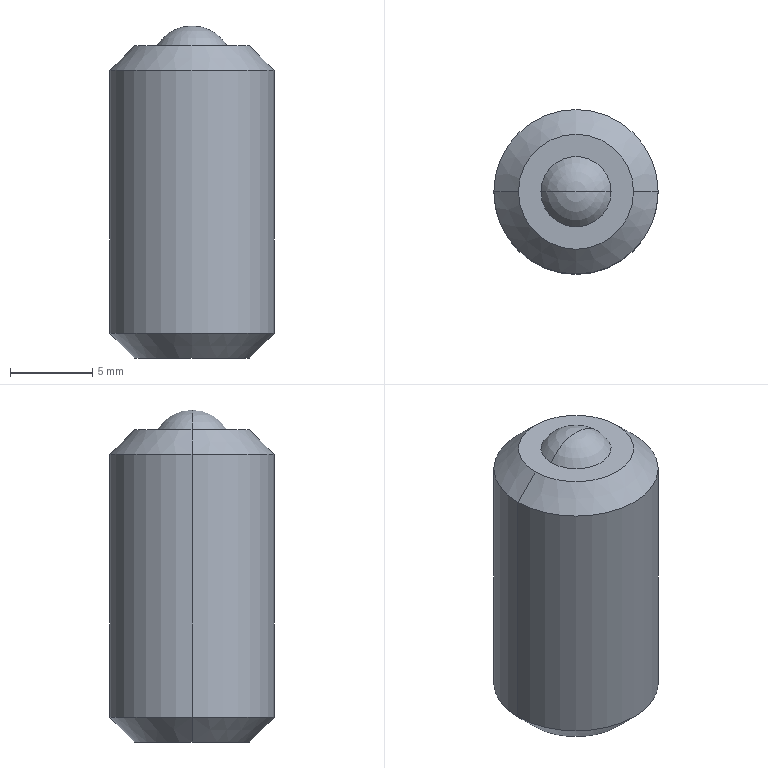Part | Creo | 1 solid | 17 faces | box 10 x 10 x 20.2 mm | volume 1251 mm3 | plane 9 | cone 4 | cylinder 2 | sphere 2 | commonest cylinder face diameters 10 x2
STEP:
#1=CARTESIAN_POINT('',(-220.5,-57.908,-54.5));
#2=VERTEX_POINT('',#1);
#3=CARTESIAN_POINT('',(-213.5,-57.908,-54.5));
#4=VERTEX_POINT('',#3);
#5=CARTESIAN_POINT('',(-217.,-57.908,-54.5));
#6=DIRECTION('',(0.,0.,-1.));
#7=DIRECTION('',(-1.,0.,0.));
#8=AXIS2_PLACEMENT_3D('',#5,#6,#7);
#9=CIRCLE('',#8,3.5);
#10=EDGE_CURVE('',#2,#4,#9,.T.);
#11=ORIENTED_EDGE('',*,*,#10,.F.);
#12=CARTESIAN_POINT('',(-217.,-57.908,-54.5));
#13=DIRECTION('',(0.,0.,-1.));
#14=DIRECTION('',(1.,0.,0.));
#15=AXIS2_PLACEMENT_3D('',#12,#13,#14);
#16=CIRCLE('',#15,3.5);
#17=EDGE_CURVE('',#4,#2,#16,.T.);
#18=ORIENTED_EDGE('',*,*,#17,.F.);
#19=EDGE_LOOP('',(#11,#18));
#20=FACE_OUTER_BOUND('',#19,.F.);
#21=CARTESIAN_POINT('',(-220.,-59.64,-54.5));
#22=VERTEX_POINT('',#21);
#23=CARTESIAN_POINT('',(-217.,-61.372,-54.5));
#24=VERTEX_POINT('',#23);
#25=CARTESIAN_POINT('',(-220.,-59.64,-54.5));
#26=DIRECTION('',(0.866,-0.5,0.));
#27=VECTOR('',#26,3.464);
#28=LINE('',#25,#27);
#29=EDGE_CURVE('',#22,#24,#28,.T.);
#30=ORIENTED_EDGE('',*,*,#29,.F.);
#31=CARTESIAN_POINT('',(-220.,-56.176,-54.5));
#32=VERTEX_POINT('',#31);
#33=CARTESIAN_POINT('',(-220.,-59.64,-54.5));
#34=DIRECTION('',(0.,1.,0.));
#35=VECTOR('',#34,3.464);
#36=LINE('',#33,#35);
#37=EDGE_CURVE('',#22,#32,#36,.T.);
#38=ORIENTED_EDGE('',*,*,#37,.T.);
#39=CARTESIAN_POINT('',(-217.,-54.444,-54.5));
#40=VERTEX_POINT('',#39);
#41=CARTESIAN_POINT('',(-217.,-54.444,-54.5));
#42=DIRECTION('',(-0.866,-0.5,0.));
#43=VECTOR('',#42,3.464);
#44=LINE('',#41,#43);
#45=EDGE_CURVE('',#40,#32,#44,.T.);
#46=ORIENTED_EDGE('',*,*,#45,.F.);
#47=CARTESIAN_POINT('',(-214.,-56.176,-54.5));
#48=VERTEX_POINT('',#47);
#49=CARTESIAN_POINT('',(-214.,-56.176,-54.5));
#50=DIRECTION('',(-0.866,0.5,0.));
#51=VECTOR('',#50,3.464);
#52=LINE('',#49,#51);
#53=EDGE_CURVE('',#48,#40,#52,.T.);
#54=ORIENTED_EDGE('',*,*,#53,.F.);
#55=CARTESIAN_POINT('',(-214.,-59.64,-54.5));
#56=VERTEX_POINT('',#55);
#57=CARTESIAN_POINT('',(-214.,-56.176,-54.5));
#58=DIRECTION('',(0.,-1.,0.));
#59=VECTOR('',#58,3.464);
#60=LINE('',#57,#59);
#61=EDGE_CURVE('',#48,#56,#60,.T.);
#62=ORIENTED_EDGE('',*,*,#61,.T.);
#63=CARTESIAN_POINT('',(-217.,-61.372,-54.5));
#64=DIRECTION('',(0.866,0.5,0.));
#65=VECTOR('',#64,3.464);
#66=LINE('',#63,#65);
#67=EDGE_CURVE('',#24,#56,#66,.T.);
#68=ORIENTED_EDGE('',*,*,#67,.F.);
#69=EDGE_LOOP('',(#30,#38,#46,#54,#62,#68));
#70=FACE_BOUND('',#69,.F.);
#71=CARTESIAN_POINT('',(-217.,-57.908,-54.5));
#72=DIRECTION('',(0.,0.,-1.));
#73=DIRECTION('',(-1.,0.,0.));
#74=AXIS2_PLACEMENT_3D('',#71,#72,#73);
#75=PLANE('',#74);
#76=ADVANCED_FACE('',(#20,#70),#75,.T.);
#77=ORIENTED_EDGE('',*,*,#10,.T.);
#78=CARTESIAN_POINT('',(-212.,-57.908,-53.));
#79=VERTEX_POINT('',#78);
#80=CARTESIAN_POINT('',(-213.5,-57.908,-54.5));
#81=DIRECTION('',(0.7071,0.,0.7071));
#82=VECTOR('',#81,2.121);
#83=LINE('',#80,#82);
#84=EDGE_CURVE('',#4,#79,#83,.T.);
#85=ORIENTED_EDGE('',*,*,#84,.T.);
#86=CARTESIAN_POINT('',(-222.,-57.908,-53.));
#87=VERTEX_POINT('',#86);
#88=CARTESIAN_POINT('',(-217.,-57.908,-53.));
#89=DIRECTION('',(0.,0.,-1.));
#90=DIRECTION('',(-1.,0.,0.));
#91=AXIS2_PLACEMENT_3D('',#88,#89,#90);
#92=CIRCLE('',#91,5.);
#93=EDGE_CURVE('',#87,#79,#92,.T.);
#94=ORIENTED_EDGE('',*,*,#93,.F.);
#95=CARTESIAN_POINT('',(-220.5,-57.908,-54.5));
#96=DIRECTION('',(-0.7071,0.,0.7071));
#97=VECTOR('',#96,2.121);
#98=LINE('',#95,#97);
#99=EDGE_CURVE('',#2,#87,#98,.T.);
#100=ORIENTED_EDGE('',*,*,#99,.F.);
#101=EDGE_LOOP('',(#77,#85,#94,#100));
#102=FACE_OUTER_BOUND('',#101,.F.);
#103=CARTESIAN_POINT('',(-217.,-57.908,-53.75));
#104=DIRECTION('',(0.,0.,1.));
#105=DIRECTION('',(1.,0.,0.));
#106=AXIS2_PLACEMENT_3D('',#103,#104,#105);
#107=CONICAL_SURFACE('',#106,4.25,45.);
#108=ADVANCED_FACE('',(#102),#107,.T.);
#109=ORIENTED_EDGE('',*,*,#17,.T.);
#110=ORIENTED_EDGE('',*,*,#99,.T.);
#111=CARTESIAN_POINT('',(-217.,-57.908,-53.));
#112=DIRECTION('',(0.,0.,-1.));
#113=DIRECTION('',(1.,0.,0.));
#114=AXIS2_PLACEMENT_3D('',#111,#112,#113);
#115=CIRCLE('',#114,5.);
#116=EDGE_CURVE('',#79,#87,#115,.T.);
#117=ORIENTED_EDGE('',*,*,#116,.F.);
#118=ORIENTED_EDGE('',*,*,#84,.F.);
#119=EDGE_LOOP('',(#109,#110,#117,#118));
#120=FACE_OUTER_BOUND('',#119,.F.);
#121=CARTESIAN_POINT('',(-217.,-57.908,-53.75));
#122=DIRECTION('',(0.,0.,1.));
#123=DIRECTION('',(1.,0.,0.));
#124=AXIS2_PLACEMENT_3D('',#121,#122,#123);
#125=CONICAL_SURFACE('',#124,4.25,45.);
#126=ADVANCED_FACE('',(#120),#125,.T.);
#127=ORIENTED_EDGE('',*,*,#116,.T.);
#128=CARTESIAN_POINT('',(-222.,-57.908,-37.));
#129=VERTEX_POINT('',#128);
#130=CARTESIAN_POINT('',(-222.,-57.908,-37.));
#131=DIRECTION('',(0.,0.,-1.));
#132=VECTOR('',#131,16.);
#133=LINE('',#130,#132);
#134=EDGE_CURVE('',#129,#87,#133,.T.);
#135=ORIENTED_EDGE('',*,*,#134,.F.);
#136=CARTESIAN_POINT('',(-212.,-57.908,-37.));
#137=VERTEX_POINT('',#136);
#138=CARTESIAN_POINT('',(-217.,-57.908,-37.));
#139=DIRECTION('',(0.,0.,1.));
#140=DIRECTION('',(-1.,0.,0.));
#141=AXIS2_PLACEMENT_3D('',#138,#139,#140);
#142=CIRCLE('',#141,5.);
#143=EDGE_CURVE('',#129,#137,#142,.T.);
#144=ORIENTED_EDGE('',*,*,#143,.T.);
#145=CARTESIAN_POINT('',(-212.,-57.908,-37.));
#146=DIRECTION('',(0.,0.,-1.));
#147=VECTOR('',#146,16.);
#148=LINE('',#145,#147);
#149=EDGE_CURVE('',#137,#79,#148,.T.);
#150=ORIENTED_EDGE('',*,*,#149,.T.);
#151=EDGE_LOOP('',(#127,#135,#144,#150));
#152=FACE_OUTER_BOUND('',#151,.F.);
#153=CARTESIAN_POINT('',(-217.,-57.908,-35.5));
#154=DIRECTION('',(0.,0.,-1.));
#155=DIRECTION('',(-1.,0.,0.));
#156=AXIS2_PLACEMENT_3D('',#153,#154,#155);
#157=CYLINDRICAL_SURFACE('',#156,5.);
#158=ADVANCED_FACE('',(#152),#157,.T.);
#159=ORIENTED_EDGE('',*,*,#93,.T.);
#160=ORIENTED_EDGE('',*,*,#149,.F.);
#161=CARTESIAN_POINT('',(-217.,-57.908,-37.));
#162=DIRECTION('',(0.,0.,1.));
#163=DIRECTION('',(1.,0.,0.));
#164=AXIS2_PLACEMENT_3D('',#161,#162,#163);
#165=CIRCLE('',#164,5.);
#166=EDGE_CURVE('',#137,#129,#165,.T.);
#167=ORIENTED_EDGE('',*,*,#166,.T.);
#168=ORIENTED_EDGE('',*,*,#134,.T.);
#169=EDGE_LOOP('',(#159,#160,#167,#168));
#170=FACE_OUTER_BOUND('',#169,.F.);
#171=CARTESIAN_POINT('',(-217.,-57.908,-35.5));
#172=DIRECTION('',(0.,0.,-1.));
#173=DIRECTION('',(-1.,0.,0.));
#174=AXIS2_PLACEMENT_3D('',#171,#172,#173);
#175=CYLINDRICAL_SURFACE('',#174,5.);
#176=ADVANCED_FACE('',(#170),#175,.T.);
#177=CARTESIAN_POINT('',(-213.5,-57.908,-35.5));
#178=VERTEX_POINT('',#177);
#179=CARTESIAN_POINT('',(-220.5,-57.908,-35.5));
#180=VERTEX_POINT('',#179);
#181=CARTESIAN_POINT('',(-217.,-57.908,-35.5));
#182=DIRECTION('',(0.,0.,1.));
#183=DIRECTION('',(1.,0.,0.));
#184=AXIS2_PLACEMENT_3D('',#181,#182,#183);
#185=CIRCLE('',#184,3.5);
#186=EDGE_CURVE('',#178,#180,#185,.T.);
#187=ORIENTED_EDGE('',*,*,#186,.T.);
#188=CARTESIAN_POINT('',(-220.5,-57.908,-35.5));
#189=DIRECTION('',(-0.7071,0.,-0.7071));
#190=VECTOR('',#189,2.121);
#191=LINE('',#188,#190);
#192=EDGE_CURVE('',#180,#129,#191,.T.);
#193=ORIENTED_EDGE('',*,*,#192,.T.);
#194=ORIENTED_EDGE('',*,*,#166,.F.);
#195=CARTESIAN_POINT('',(-213.5,-57.908,-35.5));
#196=DIRECTION('',(0.7071,0.,-0.7071));
#197=VECTOR('',#196,2.121);
#198=LINE('',#195,#197);
#199=EDGE_CURVE('',#178,#137,#198,.T.);
#200=ORIENTED_EDGE('',*,*,#199,.F.);
#201=EDGE_LOOP('',(#187,#193,#194,#200));
#202=FACE_OUTER_BOUND('',#201,.F.);
#203=CARTESIAN_POINT('',(-217.,-57.908,-36.25));
#204=DIRECTION('',(0.,0.,-1.));
#205=DIRECTION('',(-1.,0.,0.));
#206=AXIS2_PLACEMENT_3D('',#203,#204,#205);
#207=CONICAL_SURFACE('',#206,4.25,45.);
#208=ADVANCED_FACE('',(#202),#207,.T.);
#209=ORIENTED_EDGE('',*,*,#186,.F.);
#210=CARTESIAN_POINT('',(-217.,-57.908,-35.5));
#211=DIRECTION('',(0.,0.,1.));
#212=DIRECTION('',(-1.,0.,0.));
#213=AXIS2_PLACEMENT_3D('',#210,#211,#212);
#214=CIRCLE('',#213,3.5);
#215=EDGE_CURVE('',#180,#178,#214,.T.);
#216=ORIENTED_EDGE('',*,*,#215,.F.);
#217=EDGE_LOOP('',(#209,#216));
#218=FACE_OUTER_BOUND('',#217,.F.);
#219=CARTESIAN_POINT('',(-214.865,-57.908,-35.5));
#220=VERTEX_POINT('',#219);
#221=CARTESIAN_POINT('',(-219.135,-57.908,-35.5));
#222=VERTEX_POINT('',#221);
#223=CARTESIAN_POINT('',(-217.,-57.908,-35.5));
#224=DIRECTION('',(0.,0.,-1.));
#225=DIRECTION('',(1.,0.,0.));
#226=AXIS2_PLACEMENT_3D('',#223,#224,#225);
#227=CIRCLE('',#226,2.135);
#228=EDGE_CURVE('',#220,#222,#227,.T.);
#229=ORIENTED_EDGE('',*,*,#228,.F.);
#230=CARTESIAN_POINT('',(-217.,-57.908,-35.5));
#231=DIRECTION('',(0.,0.,-1.));
#232=DIRECTION('',(-1.,0.,0.));
#233=AXIS2_PLACEMENT_3D('',#230,#231,#232);
#234=CIRCLE('',#233,2.135);
#235=EDGE_CURVE('',#222,#220,#234,.T.);
#236=ORIENTED_EDGE('',*,*,#235,.F.);
#237=EDGE_LOOP('',(#229,#236));
#238=FACE_BOUND('',#237,.F.);
#239=CARTESIAN_POINT('',(-217.,-57.908,-35.5));
#240=DIRECTION('',(0.,0.,1.));
#241=DIRECTION('',(1.,0.,0.));
#242=AXIS2_PLACEMENT_3D('',#239,#240,#241);
#243=PLANE('',#242);
#244=ADVANCED_FACE('',(#218,#238),#243,.T.);
#245=ORIENTED_EDGE('',*,*,#228,.T.);
#246=CARTESIAN_POINT('',(-217.,-57.908,-34.3));
#247=VERTEX_POINT('',#246);
#248=CARTESIAN_POINT('',(-217.,-57.908,-36.8));
#249=DIRECTION('',(0.,1.,0.));
#250=DIRECTION('',(-0.8542,0.,0.52));
#251=AXIS2_PLACEMENT_3D('',#248,#249,#250);
#252=CIRCLE('',#251,2.5);
#253=EDGE_CURVE('',#222,#247,#252,.T.);
#254=ORIENTED_EDGE('',*,*,#253,.T.);
#255=CARTESIAN_POINT('',(-217.,-57.908,-36.8));
#256=DIRECTION('',(0.,-1.,0.));
#257=DIRECTION('',(0.8542,0.,0.52));
#258=AXIS2_PLACEMENT_3D('',#255,#256,#257);
#259=CIRCLE('',#258,2.5);
#260=EDGE_CURVE('',#220,#247,#259,.T.);
#261=ORIENTED_EDGE('',*,*,#260,.F.);
#262=EDGE_LOOP('',(#245,#254,#261));
#263=FACE_OUTER_BOUND('',#262,.F.);
#264=CARTESIAN_POINT('',(-217.,-57.908,-36.8));
#265=DIRECTION('',(0.,0.,1.));
#266=DIRECTION('',(1.,0.,0.));
#267=AXIS2_PLACEMENT_3D('',#264,#265,#266);
#268=SPHERICAL_SURFACE('',#267,2.5);
#269=ADVANCED_FACE('',(#263),#268,.T.);
#270=ORIENTED_EDGE('',*,*,#235,.T.);
#271=ORIENTED_EDGE('',*,*,#260,.T.);
#272=ORIENTED_EDGE('',*,*,#253,.F.);
#273=EDGE_LOOP('',(#270,#271,#272));
#274=FACE_OUTER_BOUND('',#273,.F.);
#275=CARTESIAN_POINT('',(-217.,-57.908,-36.8));
#276=DIRECTION('',(0.,0.,1.));
#277=DIRECTION('',(1.,0.,0.));
#278=AXIS2_PLACEMENT_3D('',#275,#276,#277);
#279=SPHERICAL_SURFACE('',#278,2.5);
#280=ADVANCED_FACE('',(#274),#279,.T.);
#281=ORIENTED_EDGE('',*,*,#215,.T.);
#282=ORIENTED_EDGE('',*,*,#199,.T.);
#283=ORIENTED_EDGE('',*,*,#143,.F.);
#284=ORIENTED_EDGE('',*,*,#192,.F.);
#285=EDGE_LOOP('',(#281,#282,#283,#284));
#286=FACE_OUTER_BOUND('',#285,.F.);
#287=CARTESIAN_POINT('',(-217.,-57.908,-36.25));
#288=DIRECTION('',(0.,0.,-1.));
#289=DIRECTION('',(-1.,0.,0.));
#290=AXIS2_PLACEMENT_3D('',#287,#288,#289);
#291=CONICAL_SURFACE('',#290,4.25,45.);
#292=ADVANCED_FACE('',(#286),#291,.T.);
#293=CARTESIAN_POINT('',(-217.,-61.372,-48.5));
#294=VERTEX_POINT('',#293);
#295=CARTESIAN_POINT('',(-220.,-59.64,-48.5));
#296=VERTEX_POINT('',#295);
#297=CARTESIAN_POINT('',(-217.,-61.372,-48.5));
#298=DIRECTION('',(-0.866,0.5,0.));
#299=VECTOR('',#298,3.464);
#300=LINE('',#297,#299);
#301=EDGE_CURVE('',#294,#296,#300,.T.);
#302=ORIENTED_EDGE('',*,*,#301,.T.);
#303=CARTESIAN_POINT('',(-220.,-59.64,-48.5));
#304=DIRECTION('',(0.,0.,-1.));
#305=VECTOR('',#304,6.);
#306=LINE('',#303,#305);
#307=EDGE_CURVE('',#296,#22,#306,.T.);
#308=ORIENTED_EDGE('',*,*,#307,.T.);
#309=ORIENTED_EDGE('',*,*,#29,.T.);
#310=CARTESIAN_POINT('',(-217.,-61.372,-48.5));
#311=DIRECTION('',(0.,0.,-1.));
#312=VECTOR('',#311,6.);
#313=LINE('',#310,#312);
#314=EDGE_CURVE('',#294,#24,#313,.T.);
#315=ORIENTED_EDGE('',*,*,#314,.F.);
#316=EDGE_LOOP('',(#302,#308,#309,#315));
#317=FACE_OUTER_BOUND('',#316,.F.);
#318=CARTESIAN_POINT('',(-218.5,-60.506,-51.5));
#319=DIRECTION('',(-0.5,-0.866,0.));
#320=DIRECTION('',(0.866,-0.5,0.));
#321=AXIS2_PLACEMENT_3D('',#318,#319,#320);
#322=PLANE('',#321);
#323=ADVANCED_FACE('',(#317),#322,.F.);
#324=CARTESIAN_POINT('',(-220.,-56.176,-48.5));
#325=VERTEX_POINT('',#324);
#326=CARTESIAN_POINT('',(-220.,-59.64,-48.5));
#327=DIRECTION('',(0.,1.,0.));
#328=VECTOR('',#327,3.464);
#329=LINE('',#326,#328);
#330=EDGE_CURVE('',#296,#325,#329,.T.);
#331=ORIENTED_EDGE('',*,*,#330,.F.);
#332=ORIENTED_EDGE('',*,*,#301,.F.);
#333=CARTESIAN_POINT('',(-214.,-59.64,-48.5));
#334=VERTEX_POINT('',#333);
#335=CARTESIAN_POINT('',(-214.,-59.64,-48.5));
#336=DIRECTION('',(-0.866,-0.5,0.));
#337=VECTOR('',#336,3.464);
#338=LINE('',#335,#337);
#339=EDGE_CURVE('',#334,#294,#338,.T.);
#340=ORIENTED_EDGE('',*,*,#339,.F.);
#341=CARTESIAN_POINT('',(-214.,-56.176,-48.5));
#342=VERTEX_POINT('',#341);
#343=CARTESIAN_POINT('',(-214.,-56.176,-48.5));
#344=DIRECTION('',(0.,-1.,0.));
#345=VECTOR('',#344,3.464);
#346=LINE('',#343,#345);
#347=EDGE_CURVE('',#342,#334,#346,.T.);
#348=ORIENTED_EDGE('',*,*,#347,.F.);
#349=CARTESIAN_POINT('',(-217.,-54.444,-48.5));
#350=VERTEX_POINT('',#349);
#351=CARTESIAN_POINT('',(-217.,-54.444,-48.5));
#352=DIRECTION('',(0.866,-0.5,0.));
#353=VECTOR('',#352,3.464);
#354=LINE('',#351,#353);
#355=EDGE_CURVE('',#350,#342,#354,.T.);
#356=ORIENTED_EDGE('',*,*,#355,.F.);
#357=CARTESIAN_POINT('',(-220.,-56.176,-48.5));
#358=DIRECTION('',(0.866,0.5,0.));
#359=VECTOR('',#358,3.464);
#360=LINE('',#357,#359);
#361=EDGE_CURVE('',#325,#350,#360,.T.);
#362=ORIENTED_EDGE('',*,*,#361,.F.);
#363=EDGE_LOOP('',(#331,#332,#340,#348,#356,#362));
#364=FACE_OUTER_BOUND('',#363,.F.);
#365=CARTESIAN_POINT('',(-217.,-57.908,-48.5));
#366=DIRECTION('',(0.,0.,1.));
#367=DIRECTION('',(1.,0.,0.));
#368=AXIS2_PLACEMENT_3D('',#365,#366,#367);
#369=PLANE('',#368);
#370=ADVANCED_FACE('',(#364),#369,.F.);
#371=ORIENTED_EDGE('',*,*,#330,.T.);
#372=CARTESIAN_POINT('',(-220.,-56.176,-48.5));
#373=DIRECTION('',(0.,0.,-1.));
#374=VECTOR('',#373,6.);
#375=LINE('',#372,#374);
#376=EDGE_CURVE('',#325,#32,#375,.T.);
#377=ORIENTED_EDGE('',*,*,#376,.T.);
#378=ORIENTED_EDGE('',*,*,#37,.F.);
#379=ORIENTED_EDGE('',*,*,#307,.F.);
#380=EDGE_LOOP('',(#371,#377,#378,#379));
#381=FACE_OUTER_BOUND('',#380,.F.);
#382=CARTESIAN_POINT('',(-220.,-57.908,-51.5));
#383=DIRECTION('',(-1.,0.,0.));
#384=DIRECTION('',(0.,0.,1.));
#385=AXIS2_PLACEMENT_3D('',#382,#383,#384);
#386=PLANE('',#385);
#387=ADVANCED_FACE('',(#381),#386,.F.);
#388=ORIENTED_EDGE('',*,*,#361,.T.);
#389=CARTESIAN_POINT('',(-217.,-54.444,-48.5));
#390=DIRECTION('',(0.,0.,-1.));
#391=VECTOR('',#390,6.);
#392=LINE('',#389,#391);
#393=EDGE_CURVE('',#350,#40,#392,.T.);
#394=ORIENTED_EDGE('',*,*,#393,.T.);
#395=ORIENTED_EDGE('',*,*,#45,.T.);
#396=ORIENTED_EDGE('',*,*,#376,.F.);
#397=EDGE_LOOP('',(#388,#394,#395,#396));
#398=FACE_OUTER_BOUND('',#397,.F.);
#399=CARTESIAN_POINT('',(-218.5,-55.31,-51.5));
#400=DIRECTION('',(-0.5,0.866,0.));
#401=DIRECTION('',(-0.866,-0.5,0.));
#402=AXIS2_PLACEMENT_3D('',#399,#400,#401);
#403=PLANE('',#402);
#404=ADVANCED_FACE('',(#398),#403,.F.);
#405=ORIENTED_EDGE('',*,*,#355,.T.);
#406=CARTESIAN_POINT('',(-214.,-56.176,-48.5));
#407=DIRECTION('',(0.,0.,-1.));
#408=VECTOR('',#407,6.);
#409=LINE('',#406,#408);
#410=EDGE_CURVE('',#342,#48,#409,.T.);
#411=ORIENTED_EDGE('',*,*,#410,.T.);
#412=ORIENTED_EDGE('',*,*,#53,.T.);
#413=ORIENTED_EDGE('',*,*,#393,.F.);
#414=EDGE_LOOP('',(#405,#411,#412,#413));
#415=FACE_OUTER_BOUND('',#414,.F.);
#416=CARTESIAN_POINT('',(-215.5,-55.31,-51.5));
#417=DIRECTION('',(0.5,0.866,0.));
#418=DIRECTION('',(-0.866,0.5,0.));
#419=AXIS2_PLACEMENT_3D('',#416,#417,#418);
#420=PLANE('',#419);
#421=ADVANCED_FACE('',(#415),#420,.F.);
#422=ORIENTED_EDGE('',*,*,#347,.T.);
#423=CARTESIAN_POINT('',(-214.,-59.64,-48.5));
#424=DIRECTION('',(0.,0.,-1.));
#425=VECTOR('',#424,6.);
#426=LINE('',#423,#425);
#427=EDGE_CURVE('',#334,#56,#426,.T.);
#428=ORIENTED_EDGE('',*,*,#427,.T.);
#429=ORIENTED_EDGE('',*,*,#61,.F.);
#430=ORIENTED_EDGE('',*,*,#410,.F.);
#431=EDGE_LOOP('',(#422,#428,#429,#430));
#432=FACE_OUTER_BOUND('',#431,.F.);
#433=CARTESIAN_POINT('',(-214.,-57.908,-51.5));
#434=DIRECTION('',(1.,0.,0.));
#435=DIRECTION('',(0.,0.,-1.));
#436=AXIS2_PLACEMENT_3D('',#433,#434,#435);
#437=PLANE('',#436);
#438=ADVANCED_FACE('',(#432),#437,.F.);
#439=ORIENTED_EDGE('',*,*,#339,.T.);
#440=ORIENTED_EDGE('',*,*,#314,.T.);
#441=ORIENTED_EDGE('',*,*,#67,.T.);
#442=ORIENTED_EDGE('',*,*,#427,.F.);
#443=EDGE_LOOP('',(#439,#440,#441,#442));
#444=FACE_OUTER_BOUND('',#443,.F.);
#445=CARTESIAN_POINT('',(-215.5,-60.506,-51.5));
#446=DIRECTION('',(0.5,-0.866,0.));
#447=DIRECTION('',(0.866,0.5,0.));
#448=AXIS2_PLACEMENT_3D('',#445,#446,#447);
#449=PLANE('',#448);
#450=ADVANCED_FACE('',(#444),#449,.F.);
#451=CLOSED_SHELL('',(#76,#108,#126,#158,#176,#208,#244,#269,#280,#292,#323,#370,#387,#404,#421,#438,#450));
#452=MANIFOLD_SOLID_BREP('',#451);
#453=(LENGTH_UNIT()NAMED_UNIT(*)SI_UNIT(.MILLI.,.METRE.));
#454=UNCERTAINTY_MEASURE_WITH_UNIT(LENGTH_MEASURE(0.002466),#453,'','');
#455=(NAMED_UNIT(*)PLANE_ANGLE_UNIT()SI_UNIT($,.RADIAN.));
#456=PLANE_ANGLE_MEASURE_WITH_UNIT(PLANE_ANGLE_MEASURE(0.01745),#455);
#457=(CONVERSION_BASED_UNIT('DEGREE',#456)NAMED_UNIT(*)PLANE_ANGLE_UNIT());
#458=(NAMED_UNIT(*)SI_UNIT($,.STERADIAN.)SOLID_ANGLE_UNIT());
#459=(GEOMETRIC_REPRESENTATION_CONTEXT(3)GLOBAL_UNCERTAINTY_ASSIGNED_CONTEXT((#454))GLOBAL_UNIT_ASSIGNED_CONTEXT((#453,#457,#458))REPRESENTATION_CONTEXT('',''));
#460=ADVANCED_BREP_SHAPE_REPRESENTATION('',(#452),#459);